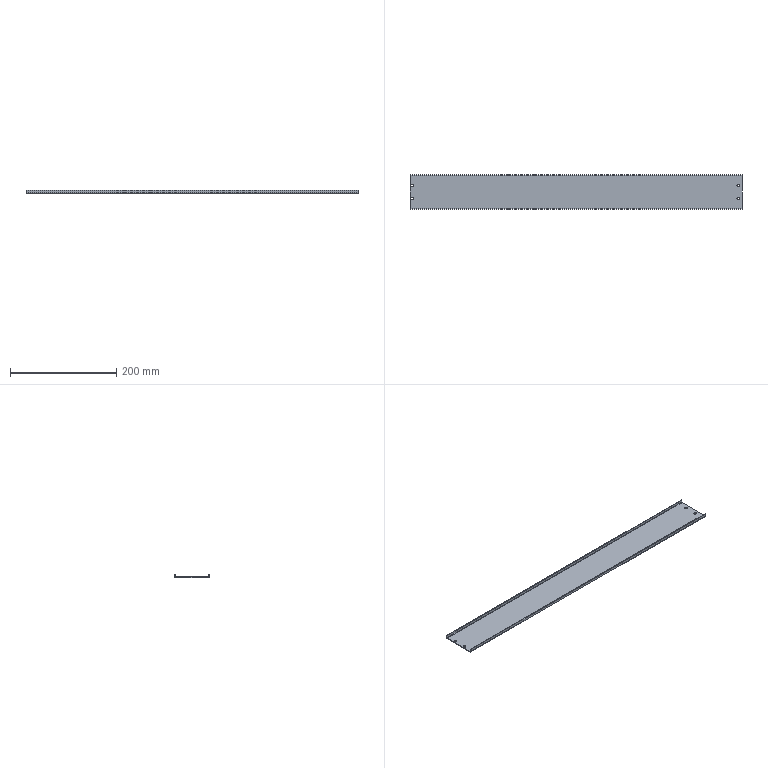Part | NX | features BREP 1 | 1 solid | 30 faces | box 625 x 65 x 6.5 mm | volume 68998 mm3 | plane 18 | cylinder 12 | commonest cylinder face diameters 5 x8 1.473 x2 4.473 x2
STEP:
#1=CARTESIAN_POINT('',(303.,-12.,0.));
#2=VERTEX_POINT('',#1);
#3=CARTESIAN_POINT('',(308.,-12.,0.));
#4=VERTEX_POINT('',#3);
#5=CARTESIAN_POINT('',(305.5,-12.,0.));
#6=DIRECTION('',(0.,0.,1.));
#7=DIRECTION('',(1.,0.,0.));
#8=AXIS2_PLACEMENT_3D('',#5,#6,#7);
#9=CIRCLE('',#8,2.5);
#10=EDGE_CURVE('',#2,#4,#9,.T.);
#11=ORIENTED_EDGE('',*,*,#10,.T.);
#12=CARTESIAN_POINT('',(308.,-12.,-1.5));
#13=VERTEX_POINT('',#12);
#14=CARTESIAN_POINT('',(308.,-12.,8.5));
#15=DIRECTION('',(0.,0.,-1.));
#16=VECTOR('',#15,1000.);
#17=LINE('',#14,#16);
#18=EDGE_CURVE('',#4,#13,#17,.T.);
#19=ORIENTED_EDGE('',*,*,#18,.T.);
#20=CARTESIAN_POINT('',(303.,-12.,-1.5));
#21=VERTEX_POINT('',#20);
#22=CARTESIAN_POINT('',(305.5,-12.,-1.5));
#23=DIRECTION('',(0.,0.,-1.));
#24=DIRECTION('',(-1.,0.,0.));
#25=AXIS2_PLACEMENT_3D('',#22,#23,#24);
#26=CIRCLE('',#25,2.5);
#27=EDGE_CURVE('',#13,#21,#26,.T.);
#28=ORIENTED_EDGE('',*,*,#27,.T.);
#29=CARTESIAN_POINT('',(303.,-12.,8.5));
#30=DIRECTION('',(0.,0.,-1.));
#31=VECTOR('',#30,1000.);
#32=LINE('',#29,#31);
#33=EDGE_CURVE('',#2,#21,#32,.T.);
#34=ORIENTED_EDGE('',*,*,#33,.F.);
#35=EDGE_LOOP('',(#11,#19,#28,#34));
#36=FACE_BOUND('',#35,.T.);
#37=CARTESIAN_POINT('',(305.5,-12.,8.5));
#38=DIRECTION('',(0.,0.,-1.));
#39=DIRECTION('',(-1.,0.,0.));
#40=AXIS2_PLACEMENT_3D('',#37,#38,#39);
#41=CYLINDRICAL_SURFACE('',#40,2.5);
#42=ADVANCED_FACE('',(#36),#41,.F.);
#43=CARTESIAN_POINT('',(303.,12.,0.));
#44=VERTEX_POINT('',#43);
#45=CARTESIAN_POINT('',(308.,12.,0.));
#46=VERTEX_POINT('',#45);
#47=CARTESIAN_POINT('',(305.5,12.,0.));
#48=DIRECTION('',(0.,0.,1.));
#49=DIRECTION('',(1.,0.,0.));
#50=AXIS2_PLACEMENT_3D('',#47,#48,#49);
#51=CIRCLE('',#50,2.5);
#52=EDGE_CURVE('',#44,#46,#51,.T.);
#53=ORIENTED_EDGE('',*,*,#52,.T.);
#54=CARTESIAN_POINT('',(308.,12.,-1.5));
#55=VERTEX_POINT('',#54);
#56=CARTESIAN_POINT('',(308.,12.,8.5));
#57=DIRECTION('',(0.,0.,-1.));
#58=VECTOR('',#57,1000.);
#59=LINE('',#56,#58);
#60=EDGE_CURVE('',#46,#55,#59,.T.);
#61=ORIENTED_EDGE('',*,*,#60,.T.);
#62=CARTESIAN_POINT('',(303.,12.,-1.5));
#63=VERTEX_POINT('',#62);
#64=CARTESIAN_POINT('',(305.5,12.,-1.5));
#65=DIRECTION('',(0.,0.,-1.));
#66=DIRECTION('',(-1.,0.,0.));
#67=AXIS2_PLACEMENT_3D('',#64,#65,#66);
#68=CIRCLE('',#67,2.5);
#69=EDGE_CURVE('',#55,#63,#68,.T.);
#70=ORIENTED_EDGE('',*,*,#69,.T.);
#71=CARTESIAN_POINT('',(303.,12.,8.5));
#72=DIRECTION('',(0.,0.,-1.));
#73=VECTOR('',#72,1000.);
#74=LINE('',#71,#73);
#75=EDGE_CURVE('',#44,#63,#74,.T.);
#76=ORIENTED_EDGE('',*,*,#75,.F.);
#77=EDGE_LOOP('',(#53,#61,#70,#76));
#78=FACE_BOUND('',#77,.T.);
#79=CARTESIAN_POINT('',(305.5,12.,8.5));
#80=DIRECTION('',(0.,0.,-1.));
#81=DIRECTION('',(-1.,0.,0.));
#82=AXIS2_PLACEMENT_3D('',#79,#80,#81);
#83=CYLINDRICAL_SURFACE('',#82,2.5);
#84=ADVANCED_FACE('',(#78),#83,.F.);
#85=CARTESIAN_POINT('',(-311.,-12.,0.));
#86=VERTEX_POINT('',#85);
#87=CARTESIAN_POINT('',(-306.,-12.,0.));
#88=VERTEX_POINT('',#87);
#89=CARTESIAN_POINT('',(-308.5,-12.,0.));
#90=DIRECTION('',(0.,0.,1.));
#91=DIRECTION('',(1.,0.,0.));
#92=AXIS2_PLACEMENT_3D('',#89,#90,#91);
#93=CIRCLE('',#92,2.5);
#94=EDGE_CURVE('',#86,#88,#93,.T.);
#95=ORIENTED_EDGE('',*,*,#94,.T.);
#96=CARTESIAN_POINT('',(-306.,-12.,-1.5));
#97=VERTEX_POINT('',#96);
#98=CARTESIAN_POINT('',(-306.,-12.,8.5));
#99=DIRECTION('',(0.,0.,-1.));
#100=VECTOR('',#99,1000.);
#101=LINE('',#98,#100);
#102=EDGE_CURVE('',#88,#97,#101,.T.);
#103=ORIENTED_EDGE('',*,*,#102,.T.);
#104=CARTESIAN_POINT('',(-311.,-12.,-1.5));
#105=VERTEX_POINT('',#104);
#106=CARTESIAN_POINT('',(-308.5,-12.,-1.5));
#107=DIRECTION('',(0.,0.,-1.));
#108=DIRECTION('',(-1.,0.,0.));
#109=AXIS2_PLACEMENT_3D('',#106,#107,#108);
#110=CIRCLE('',#109,2.5);
#111=EDGE_CURVE('',#97,#105,#110,.T.);
#112=ORIENTED_EDGE('',*,*,#111,.T.);
#113=CARTESIAN_POINT('',(-311.,-12.,8.5));
#114=DIRECTION('',(0.,0.,-1.));
#115=VECTOR('',#114,1000.);
#116=LINE('',#113,#115);
#117=EDGE_CURVE('',#86,#105,#116,.T.);
#118=ORIENTED_EDGE('',*,*,#117,.F.);
#119=EDGE_LOOP('',(#95,#103,#112,#118));
#120=FACE_BOUND('',#119,.T.);
#121=CARTESIAN_POINT('',(-308.5,-12.,8.5));
#122=DIRECTION('',(0.,0.,-1.));
#123=DIRECTION('',(-1.,0.,0.));
#124=AXIS2_PLACEMENT_3D('',#121,#122,#123);
#125=CYLINDRICAL_SURFACE('',#124,2.5);
#126=ADVANCED_FACE('',(#120),#125,.F.);
#127=CARTESIAN_POINT('',(-311.,12.,0.));
#128=VERTEX_POINT('',#127);
#129=CARTESIAN_POINT('',(-306.,12.,0.));
#130=VERTEX_POINT('',#129);
#131=CARTESIAN_POINT('',(-308.5,12.,0.));
#132=DIRECTION('',(0.,0.,1.));
#133=DIRECTION('',(1.,0.,0.));
#134=AXIS2_PLACEMENT_3D('',#131,#132,#133);
#135=CIRCLE('',#134,2.5);
#136=EDGE_CURVE('',#128,#130,#135,.T.);
#137=ORIENTED_EDGE('',*,*,#136,.T.);
#138=CARTESIAN_POINT('',(-306.,12.,-1.5));
#139=VERTEX_POINT('',#138);
#140=CARTESIAN_POINT('',(-306.,12.,8.5));
#141=DIRECTION('',(0.,0.,-1.));
#142=VECTOR('',#141,1000.);
#143=LINE('',#140,#142);
#144=EDGE_CURVE('',#130,#139,#143,.T.);
#145=ORIENTED_EDGE('',*,*,#144,.T.);
#146=CARTESIAN_POINT('',(-311.,12.,-1.5));
#147=VERTEX_POINT('',#146);
#148=CARTESIAN_POINT('',(-308.5,12.,-1.5));
#149=DIRECTION('',(0.,0.,-1.));
#150=DIRECTION('',(-1.,0.,0.));
#151=AXIS2_PLACEMENT_3D('',#148,#149,#150);
#152=CIRCLE('',#151,2.5);
#153=EDGE_CURVE('',#139,#147,#152,.T.);
#154=ORIENTED_EDGE('',*,*,#153,.T.);
#155=CARTESIAN_POINT('',(-311.,12.,8.5));
#156=DIRECTION('',(0.,0.,-1.));
#157=VECTOR('',#156,1000.);
#158=LINE('',#155,#157);
#159=EDGE_CURVE('',#128,#147,#158,.T.);
#160=ORIENTED_EDGE('',*,*,#159,.F.);
#161=EDGE_LOOP('',(#137,#145,#154,#160));
#162=FACE_BOUND('',#161,.T.);
#163=CARTESIAN_POINT('',(-308.5,12.,8.5));
#164=DIRECTION('',(0.,0.,-1.));
#165=DIRECTION('',(-1.,0.,0.));
#166=AXIS2_PLACEMENT_3D('',#163,#164,#165);
#167=CYLINDRICAL_SURFACE('',#166,2.5);
#168=ADVANCED_FACE('',(#162),#167,.F.);
#169=CARTESIAN_POINT('',(312.5,-30.263,-1.5));
#170=VERTEX_POINT('',#169);
#171=CARTESIAN_POINT('',(-312.5,-30.263,-1.5));
#172=VERTEX_POINT('',#171);
#173=CARTESIAN_POINT('',(312.5,-30.263,-1.5));
#174=DIRECTION('',(-1.,0.,0.));
#175=VECTOR('',#174,1000.);
#176=LINE('',#173,#175);
#177=EDGE_CURVE('',#170,#172,#176,.T.);
#178=ORIENTED_EDGE('',*,*,#177,.T.);
#179=CARTESIAN_POINT('',(-312.5,30.263,-1.5));
#180=VERTEX_POINT('',#179);
#181=CARTESIAN_POINT('',(-312.5,31.,-1.5));
#182=DIRECTION('',(0.,-1.,0.));
#183=VECTOR('',#182,1000.);
#184=LINE('',#181,#183);
#185=EDGE_CURVE('',#180,#172,#184,.T.);
#186=ORIENTED_EDGE('',*,*,#185,.F.);
#187=CARTESIAN_POINT('',(312.5,30.263,-1.5));
#188=VERTEX_POINT('',#187);
#189=CARTESIAN_POINT('',(-312.5,30.263,-1.5));
#190=DIRECTION('',(1.,0.,0.));
#191=VECTOR('',#190,1000.);
#192=LINE('',#189,#191);
#193=EDGE_CURVE('',#180,#188,#192,.T.);
#194=ORIENTED_EDGE('',*,*,#193,.T.);
#195=CARTESIAN_POINT('',(312.5,31.,-1.5));
#196=DIRECTION('',(0.,1.,0.));
#197=VECTOR('',#196,1000.);
#198=LINE('',#195,#197);
#199=EDGE_CURVE('',#170,#188,#198,.T.);
#200=ORIENTED_EDGE('',*,*,#199,.F.);
#201=EDGE_LOOP('',(#178,#186,#194,#200));
#202=FACE_BOUND('',#201,.T.);
#203=CARTESIAN_POINT('',(305.5,-12.,-1.5));
#204=DIRECTION('',(0.,0.,-1.));
#205=DIRECTION('',(-1.,0.,0.));
#206=AXIS2_PLACEMENT_3D('',#203,#204,#205);
#207=CIRCLE('',#206,2.5);
#208=EDGE_CURVE('',#21,#13,#207,.T.);
#209=ORIENTED_EDGE('',*,*,#208,.F.);
#210=ORIENTED_EDGE('',*,*,#27,.F.);
#211=EDGE_LOOP('',(#209,#210));
#212=FACE_BOUND('',#211,.T.);
#213=CARTESIAN_POINT('',(305.5,12.,-1.5));
#214=DIRECTION('',(0.,0.,-1.));
#215=DIRECTION('',(-1.,0.,0.));
#216=AXIS2_PLACEMENT_3D('',#213,#214,#215);
#217=CIRCLE('',#216,2.5);
#218=EDGE_CURVE('',#63,#55,#217,.T.);
#219=ORIENTED_EDGE('',*,*,#218,.F.);
#220=ORIENTED_EDGE('',*,*,#69,.F.);
#221=EDGE_LOOP('',(#219,#220));
#222=FACE_BOUND('',#221,.T.);
#223=CARTESIAN_POINT('',(-308.5,-12.,-1.5));
#224=DIRECTION('',(0.,0.,-1.));
#225=DIRECTION('',(-1.,0.,0.));
#226=AXIS2_PLACEMENT_3D('',#223,#224,#225);
#227=CIRCLE('',#226,2.5);
#228=EDGE_CURVE('',#105,#97,#227,.T.);
#229=ORIENTED_EDGE('',*,*,#228,.F.);
#230=ORIENTED_EDGE('',*,*,#111,.F.);
#231=EDGE_LOOP('',(#229,#230));
#232=FACE_BOUND('',#231,.T.);
#233=CARTESIAN_POINT('',(-308.5,12.,-1.5));
#234=DIRECTION('',(0.,0.,-1.));
#235=DIRECTION('',(-1.,0.,0.));
#236=AXIS2_PLACEMENT_3D('',#233,#234,#235);
#237=CIRCLE('',#236,2.5);
#238=EDGE_CURVE('',#147,#139,#237,.T.);
#239=ORIENTED_EDGE('',*,*,#238,.F.);
#240=ORIENTED_EDGE('',*,*,#153,.F.);
#241=EDGE_LOOP('',(#239,#240));
#242=FACE_BOUND('',#241,.T.);
#243=CARTESIAN_POINT('',(0.,0.,-1.5));
#244=DIRECTION('',(0.,0.,1.));
#245=DIRECTION('',(1.,0.,0.));
#246=AXIS2_PLACEMENT_3D('',#243,#244,#245);
#247=PLANE('',#246);
#248=ADVANCED_FACE('',(#202,#212,#222,#232,#242),#247,.F.);
#249=CARTESIAN_POINT('',(-312.5,30.263,0.));
#250=VERTEX_POINT('',#249);
#251=CARTESIAN_POINT('',(-312.5,-30.263,0.));
#252=VERTEX_POINT('',#251);
#253=CARTESIAN_POINT('',(-312.5,31.,0.));
#254=DIRECTION('',(0.,-1.,0.));
#255=VECTOR('',#254,1000.);
#256=LINE('',#253,#255);
#257=EDGE_CURVE('',#250,#252,#256,.T.);
#258=ORIENTED_EDGE('',*,*,#257,.T.);
#259=CARTESIAN_POINT('',(312.5,-30.263,0.));
#260=VERTEX_POINT('',#259);
#261=CARTESIAN_POINT('',(312.5,-30.263,0.));
#262=DIRECTION('',(-1.,0.,0.));
#263=VECTOR('',#262,1000.);
#264=LINE('',#261,#263);
#265=EDGE_CURVE('',#260,#252,#264,.T.);
#266=ORIENTED_EDGE('',*,*,#265,.F.);
#267=CARTESIAN_POINT('',(312.5,30.263,0.));
#268=VERTEX_POINT('',#267);
#269=CARTESIAN_POINT('',(312.5,31.,0.));
#270=DIRECTION('',(0.,1.,0.));
#271=VECTOR('',#270,1000.);
#272=LINE('',#269,#271);
#273=EDGE_CURVE('',#260,#268,#272,.T.);
#274=ORIENTED_EDGE('',*,*,#273,.T.);
#275=CARTESIAN_POINT('',(-312.5,30.263,0.));
#276=DIRECTION('',(1.,0.,0.));
#277=VECTOR('',#276,1000.);
#278=LINE('',#275,#277);
#279=EDGE_CURVE('',#250,#268,#278,.T.);
#280=ORIENTED_EDGE('',*,*,#279,.F.);
#281=EDGE_LOOP('',(#258,#266,#274,#280));
#282=FACE_BOUND('',#281,.T.);
#283=ORIENTED_EDGE('',*,*,#10,.F.);
#284=CARTESIAN_POINT('',(305.5,-12.,0.));
#285=DIRECTION('',(0.,0.,1.));
#286=DIRECTION('',(1.,0.,0.));
#287=AXIS2_PLACEMENT_3D('',#284,#285,#286);
#288=CIRCLE('',#287,2.5);
#289=EDGE_CURVE('',#4,#2,#288,.T.);
#290=ORIENTED_EDGE('',*,*,#289,.F.);
#291=EDGE_LOOP('',(#283,#290));
#292=FACE_BOUND('',#291,.T.);
#293=ORIENTED_EDGE('',*,*,#52,.F.);
#294=CARTESIAN_POINT('',(305.5,12.,0.));
#295=DIRECTION('',(0.,0.,1.));
#296=DIRECTION('',(1.,0.,0.));
#297=AXIS2_PLACEMENT_3D('',#294,#295,#296);
#298=CIRCLE('',#297,2.5);
#299=EDGE_CURVE('',#46,#44,#298,.T.);
#300=ORIENTED_EDGE('',*,*,#299,.F.);
#301=EDGE_LOOP('',(#293,#300));
#302=FACE_BOUND('',#301,.T.);
#303=ORIENTED_EDGE('',*,*,#94,.F.);
#304=CARTESIAN_POINT('',(-308.5,-12.,0.));
#305=DIRECTION('',(0.,0.,1.));
#306=DIRECTION('',(1.,0.,0.));
#307=AXIS2_PLACEMENT_3D('',#304,#305,#306);
#308=CIRCLE('',#307,2.5);
#309=EDGE_CURVE('',#88,#86,#308,.T.);
#310=ORIENTED_EDGE('',*,*,#309,.F.);
#311=EDGE_LOOP('',(#303,#310));
#312=FACE_BOUND('',#311,.T.);
#313=ORIENTED_EDGE('',*,*,#136,.F.);
#314=CARTESIAN_POINT('',(-308.5,12.,0.));
#315=DIRECTION('',(0.,0.,1.));
#316=DIRECTION('',(1.,0.,0.));
#317=AXIS2_PLACEMENT_3D('',#314,#315,#316);
#318=CIRCLE('',#317,2.5);
#319=EDGE_CURVE('',#130,#128,#318,.T.);
#320=ORIENTED_EDGE('',*,*,#319,.F.);
#321=EDGE_LOOP('',(#313,#320));
#322=FACE_BOUND('',#321,.T.);
#323=CARTESIAN_POINT('',(0.,0.,0.));
#324=DIRECTION('',(0.,0.,1.));
#325=DIRECTION('',(1.,0.,0.));
#326=AXIS2_PLACEMENT_3D('',#323,#324,#325);
#327=PLANE('',#326);
#328=ADVANCED_FACE('',(#282,#292,#302,#312,#322),#327,.T.);
#329=ORIENTED_EDGE('',*,*,#273,.F.);
#330=CARTESIAN_POINT('',(312.5,-30.263,0.));
#331=DIRECTION('',(0.,0.,-1.));
#332=VECTOR('',#331,1000.);
#333=LINE('',#330,#332);
#334=EDGE_CURVE('',#260,#170,#333,.T.);
#335=ORIENTED_EDGE('',*,*,#334,.T.);
#336=ORIENTED_EDGE('',*,*,#199,.T.);
#337=CARTESIAN_POINT('',(312.5,30.263,0.));
#338=DIRECTION('',(0.,0.,-1.));
#339=VECTOR('',#338,1000.);
#340=LINE('',#337,#339);
#341=EDGE_CURVE('',#268,#188,#340,.T.);
#342=ORIENTED_EDGE('',*,*,#341,.F.);
#343=EDGE_LOOP('',(#329,#335,#336,#342));
#344=FACE_BOUND('',#343,.T.);
#345=CARTESIAN_POINT('',(312.5,31.,-1.5));
#346=DIRECTION('',(1.,0.,0.));
#347=DIRECTION('',(0.,1.,0.));
#348=AXIS2_PLACEMENT_3D('',#345,#346,#347);
#349=PLANE('',#348);
#350=ADVANCED_FACE('',(#344),#349,.T.);
#351=CARTESIAN_POINT('',(-312.5,-30.263,0.));
#352=DIRECTION('',(0.,0.,-1.));
#353=VECTOR('',#352,1000.);
#354=LINE('',#351,#353);
#355=EDGE_CURVE('',#252,#172,#354,.T.);
#356=ORIENTED_EDGE('',*,*,#355,.F.);
#357=ORIENTED_EDGE('',*,*,#257,.F.);
#358=CARTESIAN_POINT('',(-312.5,30.263,0.));
#359=DIRECTION('',(0.,0.,-1.));
#360=VECTOR('',#359,1000.);
#361=LINE('',#358,#360);
#362=EDGE_CURVE('',#250,#180,#361,.T.);
#363=ORIENTED_EDGE('',*,*,#362,.T.);
#364=ORIENTED_EDGE('',*,*,#185,.T.);
#365=EDGE_LOOP('',(#356,#357,#363,#364));
#366=FACE_BOUND('',#365,.T.);
#367=CARTESIAN_POINT('',(-312.5,31.,-1.5));
#368=DIRECTION('',(-1.,0.,0.));
#369=DIRECTION('',(0.,0.,1.));
#370=AXIS2_PLACEMENT_3D('',#367,#368,#369);
#371=PLANE('',#370);
#372=ADVANCED_FACE('',(#366),#371,.T.);
#373=CARTESIAN_POINT('',(312.5,31.,0.7366));
#374=VERTEX_POINT('',#373);
#375=CARTESIAN_POINT('',(312.5,32.5,0.7366));
#376=VERTEX_POINT('',#375);
#377=CARTESIAN_POINT('',(312.5,31.,0.7366));
#378=DIRECTION('',(0.,1.,0.));
#379=VECTOR('',#378,1000.);
#380=LINE('',#377,#379);
#381=EDGE_CURVE('',#374,#376,#380,.T.);
#382=ORIENTED_EDGE('',*,*,#381,.F.);
#383=CARTESIAN_POINT('',(312.5,30.263,0.7366));
#384=DIRECTION('',(1.,0.,0.));
#385=DIRECTION('',(0.,0.,1.));
#386=AXIS2_PLACEMENT_3D('',#383,#384,#385);
#387=CIRCLE('',#386,0.7366);
#388=EDGE_CURVE('',#268,#374,#387,.T.);
#389=ORIENTED_EDGE('',*,*,#388,.F.);
#390=ORIENTED_EDGE('',*,*,#341,.T.);
#391=CARTESIAN_POINT('',(312.5,30.263,0.7366));
#392=DIRECTION('',(1.,0.,0.));
#393=DIRECTION('',(0.,0.,1.));
#394=AXIS2_PLACEMENT_3D('',#391,#392,#393);
#395=CIRCLE('',#394,2.237);
#396=EDGE_CURVE('',#188,#376,#395,.T.);
#397=ORIENTED_EDGE('',*,*,#396,.T.);
#398=EDGE_LOOP('',(#382,#389,#390,#397));
#399=FACE_BOUND('',#398,.T.);
#400=CARTESIAN_POINT('',(312.5,30.263,0.7366));
#401=DIRECTION('',(1.,0.,0.));
#402=DIRECTION('',(0.,1.,0.));
#403=AXIS2_PLACEMENT_3D('',#400,#401,#402);
#404=PLANE('',#403);
#405=ADVANCED_FACE('',(#399),#404,.T.);
#406=CARTESIAN_POINT('',(-312.5,31.,0.7366));
#407=VERTEX_POINT('',#406);
#408=CARTESIAN_POINT('',(-312.5,30.263,0.7366));
#409=DIRECTION('',(-1.,0.,0.));
#410=DIRECTION('',(0.,0.,1.));
#411=AXIS2_PLACEMENT_3D('',#408,#409,#410);
#412=CIRCLE('',#411,0.7366);
#413=EDGE_CURVE('',#407,#250,#412,.T.);
#414=ORIENTED_EDGE('',*,*,#413,.F.);
#415=CARTESIAN_POINT('',(-312.5,32.5,0.7366));
#416=VERTEX_POINT('',#415);
#417=CARTESIAN_POINT('',(-312.5,31.,0.7366));
#418=DIRECTION('',(0.,1.,0.));
#419=VECTOR('',#418,1000.);
#420=LINE('',#417,#419);
#421=EDGE_CURVE('',#407,#416,#420,.T.);
#422=ORIENTED_EDGE('',*,*,#421,.T.);
#423=CARTESIAN_POINT('',(-312.5,30.263,0.7366));
#424=DIRECTION('',(-1.,0.,0.));
#425=DIRECTION('',(0.,0.,1.));
#426=AXIS2_PLACEMENT_3D('',#423,#424,#425);
#427=CIRCLE('',#426,2.237);
#428=EDGE_CURVE('',#416,#180,#427,.T.);
#429=ORIENTED_EDGE('',*,*,#428,.T.);
#430=ORIENTED_EDGE('',*,*,#362,.F.);
#431=EDGE_LOOP('',(#414,#422,#429,#430));
#432=FACE_BOUND('',#431,.T.);
#433=CARTESIAN_POINT('',(-312.5,30.263,0.7366));
#434=DIRECTION('',(1.,0.,0.));
#435=DIRECTION('',(0.,1.,0.));
#436=AXIS2_PLACEMENT_3D('',#433,#434,#435);
#437=PLANE('',#436);
#438=ADVANCED_FACE('',(#432),#437,.F.);
#439=ORIENTED_EDGE('',*,*,#193,.F.);
#440=ORIENTED_EDGE('',*,*,#428,.F.);
#441=CARTESIAN_POINT('',(0.,32.5,0.7366));
#442=DIRECTION('',(-1.,0.,0.));
#443=VECTOR('',#442,1000.);
#444=LINE('',#441,#443);
#445=EDGE_CURVE('',#376,#416,#444,.T.);
#446=ORIENTED_EDGE('',*,*,#445,.F.);
#447=ORIENTED_EDGE('',*,*,#396,.F.);
#448=EDGE_LOOP('',(#439,#440,#446,#447));
#449=FACE_BOUND('',#448,.T.);
#450=CARTESIAN_POINT('',(-312.5,30.263,0.7366));
#451=DIRECTION('',(-1.,0.,0.));
#452=DIRECTION('',(0.,1.,0.));
#453=AXIS2_PLACEMENT_3D('',#450,#451,#452);
#454=CYLINDRICAL_SURFACE('',#453,2.237);
#455=ADVANCED_FACE('',(#449),#454,.T.);
#456=ORIENTED_EDGE('',*,*,#279,.T.);
#457=ORIENTED_EDGE('',*,*,#388,.T.);
#458=CARTESIAN_POINT('',(312.5,31.,0.7366));
#459=DIRECTION('',(-1.,0.,0.));
#460=VECTOR('',#459,1000.);
#461=LINE('',#458,#460);
#462=EDGE_CURVE('',#374,#407,#461,.T.);
#463=ORIENTED_EDGE('',*,*,#462,.T.);
#464=ORIENTED_EDGE('',*,*,#413,.T.);
#465=EDGE_LOOP('',(#456,#457,#463,#464));
#466=FACE_BOUND('',#465,.T.);
#467=CARTESIAN_POINT('',(-312.5,30.263,0.7366));
#468=DIRECTION('',(-1.,0.,0.));
#469=DIRECTION('',(0.,1.,0.));
#470=AXIS2_PLACEMENT_3D('',#467,#468,#469);
#471=CYLINDRICAL_SURFACE('',#470,0.7366);
#472=ADVANCED_FACE('',(#466),#471,.F.);
#473=CARTESIAN_POINT('',(-312.5,32.5,5.));
#474=VERTEX_POINT('',#473);
#475=CARTESIAN_POINT('',(-312.5,32.5,0.));
#476=DIRECTION('',(0.,0.,-1.));
#477=VECTOR('',#476,1000.);
#478=LINE('',#475,#477);
#479=EDGE_CURVE('',#474,#416,#478,.T.);
#480=ORIENTED_EDGE('',*,*,#479,.T.);
#481=ORIENTED_EDGE('',*,*,#421,.F.);
#482=CARTESIAN_POINT('',(-312.5,31.,5.));
#483=VERTEX_POINT('',#482);
#484=CARTESIAN_POINT('',(-312.5,31.,0.));
#485=DIRECTION('',(0.,0.,-1.));
#486=VECTOR('',#485,1000.);
#487=LINE('',#484,#486);
#488=EDGE_CURVE('',#483,#407,#487,.T.);
#489=ORIENTED_EDGE('',*,*,#488,.F.);
#490=CARTESIAN_POINT('',(-312.5,32.5,5.));
#491=DIRECTION('',(0.,-1.,0.));
#492=VECTOR('',#491,1000.);
#493=LINE('',#490,#492);
#494=EDGE_CURVE('',#474,#483,#493,.T.);
#495=ORIENTED_EDGE('',*,*,#494,.F.);
#496=EDGE_LOOP('',(#480,#481,#489,#495));
#497=FACE_BOUND('',#496,.T.);
#498=CARTESIAN_POINT('',(-312.5,32.5,0.));
#499=DIRECTION('',(-1.,0.,0.));
#500=DIRECTION('',(0.,0.,1.));
#501=AXIS2_PLACEMENT_3D('',#498,#499,#500);
#502=PLANE('',#501);
#503=ADVANCED_FACE('',(#497),#502,.T.);
#504=CARTESIAN_POINT('',(312.5,31.,5.));
#505=VERTEX_POINT('',#504);
#506=CARTESIAN_POINT('',(312.5,31.,5.));
#507=DIRECTION('',(0.,0.,1.));
#508=VECTOR('',#507,1000.);
#509=LINE('',#506,#508);
#510=EDGE_CURVE('',#374,#505,#509,.T.);
#511=ORIENTED_EDGE('',*,*,#510,.F.);
#512=ORIENTED_EDGE('',*,*,#381,.T.);
#513=CARTESIAN_POINT('',(312.5,32.5,5.));
#514=VERTEX_POINT('',#513);
#515=CARTESIAN_POINT('',(312.5,32.5,5.));
#516=DIRECTION('',(0.,0.,1.));
#517=VECTOR('',#516,1000.);
#518=LINE('',#515,#517);
#519=EDGE_CURVE('',#376,#514,#518,.T.);
#520=ORIENTED_EDGE('',*,*,#519,.T.);
#521=CARTESIAN_POINT('',(312.5,32.5,5.));
#522=DIRECTION('',(0.,-1.,0.));
#523=VECTOR('',#522,1000.);
#524=LINE('',#521,#523);
#525=EDGE_CURVE('',#514,#505,#524,.T.);
#526=ORIENTED_EDGE('',*,*,#525,.T.);
#527=EDGE_LOOP('',(#511,#512,#520,#526));
#528=FACE_BOUND('',#527,.T.);
#529=CARTESIAN_POINT('',(312.5,32.5,5.));
#530=DIRECTION('',(1.,0.,0.));
#531=DIRECTION('',(0.,1.,0.));
#532=AXIS2_PLACEMENT_3D('',#529,#530,#531);
#533=PLANE('',#532);
#534=ADVANCED_FACE('',(#528),#533,.T.);
#535=ORIENTED_EDGE('',*,*,#519,.F.);
#536=ORIENTED_EDGE('',*,*,#445,.T.);
#537=ORIENTED_EDGE('',*,*,#479,.F.);
#538=CARTESIAN_POINT('',(-312.5,32.5,5.));
#539=DIRECTION('',(-1.,0.,0.));
#540=VECTOR('',#539,1000.);
#541=LINE('',#538,#540);
#542=EDGE_CURVE('',#514,#474,#541,.T.);
#543=ORIENTED_EDGE('',*,*,#542,.F.);
#544=EDGE_LOOP('',(#535,#536,#537,#543));
#545=FACE_BOUND('',#544,.T.);
#546=CARTESIAN_POINT('',(0.,32.5,0.));
#547=DIRECTION('',(0.,1.,0.));
#548=DIRECTION('',(0.,0.,-1.));
#549=AXIS2_PLACEMENT_3D('',#546,#547,#548);
#550=PLANE('',#549);
#551=ADVANCED_FACE('',(#545),#550,.T.);
#552=ORIENTED_EDGE('',*,*,#462,.F.);
#553=ORIENTED_EDGE('',*,*,#510,.T.);
#554=CARTESIAN_POINT('',(-312.5,31.,5.));
#555=DIRECTION('',(-1.,0.,0.));
#556=VECTOR('',#555,1000.);
#557=LINE('',#554,#556);
#558=EDGE_CURVE('',#505,#483,#557,.T.);
#559=ORIENTED_EDGE('',*,*,#558,.T.);
#560=ORIENTED_EDGE('',*,*,#488,.T.);
#561=EDGE_LOOP('',(#552,#553,#559,#560));
#562=FACE_BOUND('',#561,.T.);
#563=CARTESIAN_POINT('',(0.,31.,0.));
#564=DIRECTION('',(0.,1.,0.));
#565=DIRECTION('',(0.,0.,-1.));
#566=AXIS2_PLACEMENT_3D('',#563,#564,#565);
#567=PLANE('',#566);
#568=ADVANCED_FACE('',(#562),#567,.F.);
#569=ORIENTED_EDGE('',*,*,#558,.F.);
#570=ORIENTED_EDGE('',*,*,#525,.F.);
#571=ORIENTED_EDGE('',*,*,#542,.T.);
#572=ORIENTED_EDGE('',*,*,#494,.T.);
#573=EDGE_LOOP('',(#569,#570,#571,#572));
#574=FACE_BOUND('',#573,.T.);
#575=CARTESIAN_POINT('',(-312.5,32.5,5.));
#576=DIRECTION('',(0.,0.,1.));
#577=DIRECTION('',(0.,-1.,0.));
#578=AXIS2_PLACEMENT_3D('',#575,#576,#577);
#579=PLANE('',#578);
#580=ADVANCED_FACE('',(#574),#579,.T.);
#581=CARTESIAN_POINT('',(-312.5,-31.,0.7366));
#582=VERTEX_POINT('',#581);
#583=CARTESIAN_POINT('',(-312.5,-32.5,0.7366));
#584=VERTEX_POINT('',#583);
#585=CARTESIAN_POINT('',(-312.5,-31.,0.7366));
#586=DIRECTION('',(0.,-1.,0.));
#587=VECTOR('',#586,1000.);
#588=LINE('',#585,#587);
#589=EDGE_CURVE('',#582,#584,#588,.T.);
#590=ORIENTED_EDGE('',*,*,#589,.F.);
#591=CARTESIAN_POINT('',(-312.5,-30.263,0.7366));
#592=DIRECTION('',(-1.,0.,0.));
#593=DIRECTION('',(0.,0.,-1.));
#594=AXIS2_PLACEMENT_3D('',#591,#592,#593);
#595=CIRCLE('',#594,0.7366);
#596=EDGE_CURVE('',#252,#582,#595,.T.);
#597=ORIENTED_EDGE('',*,*,#596,.F.);
#598=ORIENTED_EDGE('',*,*,#355,.T.);
#599=CARTESIAN_POINT('',(-312.5,-30.263,0.7366));
#600=DIRECTION('',(-1.,0.,0.));
#601=DIRECTION('',(0.,0.,-1.));
#602=AXIS2_PLACEMENT_3D('',#599,#600,#601);
#603=CIRCLE('',#602,2.237);
#604=EDGE_CURVE('',#172,#584,#603,.T.);
#605=ORIENTED_EDGE('',*,*,#604,.T.);
#606=EDGE_LOOP('',(#590,#597,#598,#605));
#607=FACE_BOUND('',#606,.T.);
#608=CARTESIAN_POINT('',(-312.5,-30.263,0.7366));
#609=DIRECTION('',(-1.,0.,0.));
#610=DIRECTION('',(0.,0.,1.));
#611=AXIS2_PLACEMENT_3D('',#608,#609,#610);
#612=PLANE('',#611);
#613=ADVANCED_FACE('',(#607),#612,.T.);
#614=CARTESIAN_POINT('',(312.5,-31.,0.7366));
#615=VERTEX_POINT('',#614);
#616=CARTESIAN_POINT('',(312.5,-30.263,0.7366));
#617=DIRECTION('',(1.,0.,0.));
#618=DIRECTION('',(0.,0.,-1.));
#619=AXIS2_PLACEMENT_3D('',#616,#617,#618);
#620=CIRCLE('',#619,0.7366);
#621=EDGE_CURVE('',#615,#260,#620,.T.);
#622=ORIENTED_EDGE('',*,*,#621,.F.);
#623=CARTESIAN_POINT('',(312.5,-32.5,0.7366));
#624=VERTEX_POINT('',#623);
#625=CARTESIAN_POINT('',(312.5,-31.,0.7366));
#626=DIRECTION('',(0.,-1.,0.));
#627=VECTOR('',#626,1000.);
#628=LINE('',#625,#627);
#629=EDGE_CURVE('',#615,#624,#628,.T.);
#630=ORIENTED_EDGE('',*,*,#629,.T.);
#631=CARTESIAN_POINT('',(312.5,-30.263,0.7366));
#632=DIRECTION('',(1.,0.,0.));
#633=DIRECTION('',(0.,0.,-1.));
#634=AXIS2_PLACEMENT_3D('',#631,#632,#633);
#635=CIRCLE('',#634,2.237);
#636=EDGE_CURVE('',#624,#170,#635,.T.);
#637=ORIENTED_EDGE('',*,*,#636,.T.);
#638=ORIENTED_EDGE('',*,*,#334,.F.);
#639=EDGE_LOOP('',(#622,#630,#637,#638));
#640=FACE_BOUND('',#639,.T.);
#641=CARTESIAN_POINT('',(312.5,-30.263,0.7366));
#642=DIRECTION('',(-1.,0.,0.));
#643=DIRECTION('',(0.,0.,1.));
#644=AXIS2_PLACEMENT_3D('',#641,#642,#643);
#645=PLANE('',#644);
#646=ADVANCED_FACE('',(#640),#645,.F.);
#647=ORIENTED_EDGE('',*,*,#177,.F.);
#648=ORIENTED_EDGE('',*,*,#636,.F.);
#649=CARTESIAN_POINT('',(0.,-32.5,0.7366));
#650=DIRECTION('',(-1.,0.,0.));
#651=VECTOR('',#650,1000.);
#652=LINE('',#649,#651);
#653=EDGE_CURVE('',#624,#584,#652,.T.);
#654=ORIENTED_EDGE('',*,*,#653,.T.);
#655=ORIENTED_EDGE('',*,*,#604,.F.);
#656=EDGE_LOOP('',(#647,#648,#654,#655));
#657=FACE_BOUND('',#656,.T.);
#658=CARTESIAN_POINT('',(312.5,-30.263,0.7366));
#659=DIRECTION('',(1.,0.,0.));
#660=DIRECTION('',(0.,-1.,0.));
#661=AXIS2_PLACEMENT_3D('',#658,#659,#660);
#662=CYLINDRICAL_SURFACE('',#661,2.237);
#663=ADVANCED_FACE('',(#657),#662,.T.);
#664=ORIENTED_EDGE('',*,*,#265,.T.);
#665=ORIENTED_EDGE('',*,*,#596,.T.);
#666=CARTESIAN_POINT('',(-312.5,-31.,0.7366));
#667=DIRECTION('',(1.,0.,0.));
#668=VECTOR('',#667,1000.);
#669=LINE('',#666,#668);
#670=EDGE_CURVE('',#582,#615,#669,.T.);
#671=ORIENTED_EDGE('',*,*,#670,.T.);
#672=ORIENTED_EDGE('',*,*,#621,.T.);
#673=EDGE_LOOP('',(#664,#665,#671,#672));
#674=FACE_BOUND('',#673,.T.);
#675=CARTESIAN_POINT('',(312.5,-30.263,0.7366));
#676=DIRECTION('',(1.,0.,0.));
#677=DIRECTION('',(0.,-1.,0.));
#678=AXIS2_PLACEMENT_3D('',#675,#676,#677);
#679=CYLINDRICAL_SURFACE('',#678,0.7366);
#680=ADVANCED_FACE('',(#674),#679,.F.);
#681=CARTESIAN_POINT('',(-312.5,-31.,5.));
#682=VERTEX_POINT('',#681);
#683=CARTESIAN_POINT('',(-312.5,-31.,0.));
#684=DIRECTION('',(0.,0.,1.));
#685=VECTOR('',#684,1000.);
#686=LINE('',#683,#685);
#687=EDGE_CURVE('',#582,#682,#686,.T.);
#688=ORIENTED_EDGE('',*,*,#687,.F.);
#689=ORIENTED_EDGE('',*,*,#589,.T.);
#690=CARTESIAN_POINT('',(-312.5,-32.5,5.));
#691=VERTEX_POINT('',#690);
#692=CARTESIAN_POINT('',(-312.5,-32.5,0.));
#693=DIRECTION('',(0.,0.,1.));
#694=VECTOR('',#693,1000.);
#695=LINE('',#692,#694);
#696=EDGE_CURVE('',#584,#691,#695,.T.);
#697=ORIENTED_EDGE('',*,*,#696,.T.);
#698=CARTESIAN_POINT('',(-312.5,-32.5,5.));
#699=DIRECTION('',(0.,1.,0.));
#700=VECTOR('',#699,1000.);
#701=LINE('',#698,#700);
#702=EDGE_CURVE('',#691,#682,#701,.T.);
#703=ORIENTED_EDGE('',*,*,#702,.T.);
#704=EDGE_LOOP('',(#688,#689,#697,#703));
#705=FACE_BOUND('',#704,.T.);
#706=CARTESIAN_POINT('',(-312.5,-32.5,0.));
#707=DIRECTION('',(-1.,0.,0.));
#708=DIRECTION('',(0.,0.,1.));
#709=AXIS2_PLACEMENT_3D('',#706,#707,#708);
#710=PLANE('',#709);
#711=ADVANCED_FACE('',(#705),#710,.T.);
#712=CARTESIAN_POINT('',(312.5,-32.5,5.));
#713=VERTEX_POINT('',#712);
#714=CARTESIAN_POINT('',(312.5,-32.5,5.));
#715=DIRECTION('',(0.,0.,-1.));
#716=VECTOR('',#715,1000.);
#717=LINE('',#714,#716);
#718=EDGE_CURVE('',#713,#624,#717,.T.);
#719=ORIENTED_EDGE('',*,*,#718,.T.);
#720=ORIENTED_EDGE('',*,*,#629,.F.);
#721=CARTESIAN_POINT('',(312.5,-31.,5.));
#722=VERTEX_POINT('',#721);
#723=CARTESIAN_POINT('',(312.5,-31.,5.));
#724=DIRECTION('',(0.,0.,-1.));
#725=VECTOR('',#724,1000.);
#726=LINE('',#723,#725);
#727=EDGE_CURVE('',#722,#615,#726,.T.);
#728=ORIENTED_EDGE('',*,*,#727,.F.);
#729=CARTESIAN_POINT('',(312.5,-32.5,5.));
#730=DIRECTION('',(0.,1.,0.));
#731=VECTOR('',#730,1000.);
#732=LINE('',#729,#731);
#733=EDGE_CURVE('',#713,#722,#732,.T.);
#734=ORIENTED_EDGE('',*,*,#733,.F.);
#735=EDGE_LOOP('',(#719,#720,#728,#734));
#736=FACE_BOUND('',#735,.T.);
#737=CARTESIAN_POINT('',(312.5,-32.5,5.));
#738=DIRECTION('',(1.,0.,0.));
#739=DIRECTION('',(0.,1.,0.));
#740=AXIS2_PLACEMENT_3D('',#737,#738,#739);
#741=PLANE('',#740);
#742=ADVANCED_FACE('',(#736),#741,.T.);
#743=ORIENTED_EDGE('',*,*,#653,.F.);
#744=ORIENTED_EDGE('',*,*,#718,.F.);
#745=CARTESIAN_POINT('',(-312.5,-32.5,5.));
#746=DIRECTION('',(1.,0.,0.));
#747=VECTOR('',#746,1000.);
#748=LINE('',#745,#747);
#749=EDGE_CURVE('',#691,#713,#748,.T.);
#750=ORIENTED_EDGE('',*,*,#749,.F.);
#751=ORIENTED_EDGE('',*,*,#696,.F.);
#752=EDGE_LOOP('',(#743,#744,#750,#751));
#753=FACE_BOUND('',#752,.T.);
#754=CARTESIAN_POINT('',(0.,-32.5,0.));
#755=DIRECTION('',(0.,1.,0.));
#756=DIRECTION('',(0.,0.,-1.));
#757=AXIS2_PLACEMENT_3D('',#754,#755,#756);
#758=PLANE('',#757);
#759=ADVANCED_FACE('',(#753),#758,.F.);
#760=ORIENTED_EDGE('',*,*,#727,.T.);
#761=ORIENTED_EDGE('',*,*,#670,.F.);
#762=ORIENTED_EDGE('',*,*,#687,.T.);
#763=CARTESIAN_POINT('',(-312.5,-31.,5.));
#764=DIRECTION('',(1.,0.,0.));
#765=VECTOR('',#764,1000.);
#766=LINE('',#763,#765);
#767=EDGE_CURVE('',#682,#722,#766,.T.);
#768=ORIENTED_EDGE('',*,*,#767,.T.);
#769=EDGE_LOOP('',(#760,#761,#762,#768));
#770=FACE_BOUND('',#769,.T.);
#771=CARTESIAN_POINT('',(0.,-31.,0.));
#772=DIRECTION('',(0.,1.,0.));
#773=DIRECTION('',(0.,0.,-1.));
#774=AXIS2_PLACEMENT_3D('',#771,#772,#773);
#775=PLANE('',#774);
#776=ADVANCED_FACE('',(#770),#775,.T.);
#777=ORIENTED_EDGE('',*,*,#767,.F.);
#778=ORIENTED_EDGE('',*,*,#702,.F.);
#779=ORIENTED_EDGE('',*,*,#749,.T.);
#780=ORIENTED_EDGE('',*,*,#733,.T.);
#781=EDGE_LOOP('',(#777,#778,#779,#780));
#782=FACE_BOUND('',#781,.T.);
#783=CARTESIAN_POINT('',(-312.5,-32.5,5.));
#784=DIRECTION('',(0.,0.,1.));
#785=DIRECTION('',(0.,-1.,0.));
#786=AXIS2_PLACEMENT_3D('',#783,#784,#785);
#787=PLANE('',#786);
#788=ADVANCED_FACE('',(#782),#787,.T.);
#789=ORIENTED_EDGE('',*,*,#144,.F.);
#790=ORIENTED_EDGE('',*,*,#319,.T.);
#791=ORIENTED_EDGE('',*,*,#159,.T.);
#792=ORIENTED_EDGE('',*,*,#238,.T.);
#793=EDGE_LOOP('',(#789,#790,#791,#792));
#794=FACE_BOUND('',#793,.T.);
#795=CARTESIAN_POINT('',(-308.5,12.,8.5));
#796=DIRECTION('',(0.,0.,-1.));
#797=DIRECTION('',(-1.,0.,0.));
#798=AXIS2_PLACEMENT_3D('',#795,#796,#797);
#799=CYLINDRICAL_SURFACE('',#798,2.5);
#800=ADVANCED_FACE('',(#794),#799,.F.);
#801=ORIENTED_EDGE('',*,*,#102,.F.);
#802=ORIENTED_EDGE('',*,*,#309,.T.);
#803=ORIENTED_EDGE('',*,*,#117,.T.);
#804=ORIENTED_EDGE('',*,*,#228,.T.);
#805=EDGE_LOOP('',(#801,#802,#803,#804));
#806=FACE_BOUND('',#805,.T.);
#807=CARTESIAN_POINT('',(-308.5,-12.,8.5));
#808=DIRECTION('',(0.,0.,-1.));
#809=DIRECTION('',(-1.,0.,0.));
#810=AXIS2_PLACEMENT_3D('',#807,#808,#809);
#811=CYLINDRICAL_SURFACE('',#810,2.5);
#812=ADVANCED_FACE('',(#806),#811,.F.);
#813=ORIENTED_EDGE('',*,*,#60,.F.);
#814=ORIENTED_EDGE('',*,*,#299,.T.);
#815=ORIENTED_EDGE('',*,*,#75,.T.);
#816=ORIENTED_EDGE('',*,*,#218,.T.);
#817=EDGE_LOOP('',(#813,#814,#815,#816));
#818=FACE_BOUND('',#817,.T.);
#819=CARTESIAN_POINT('',(305.5,12.,8.5));
#820=DIRECTION('',(0.,0.,-1.));
#821=DIRECTION('',(-1.,0.,0.));
#822=AXIS2_PLACEMENT_3D('',#819,#820,#821);
#823=CYLINDRICAL_SURFACE('',#822,2.5);
#824=ADVANCED_FACE('',(#818),#823,.F.);
#825=ORIENTED_EDGE('',*,*,#18,.F.);
#826=ORIENTED_EDGE('',*,*,#289,.T.);
#827=ORIENTED_EDGE('',*,*,#33,.T.);
#828=ORIENTED_EDGE('',*,*,#208,.T.);
#829=EDGE_LOOP('',(#825,#826,#827,#828));
#830=FACE_BOUND('',#829,.T.);
#831=CARTESIAN_POINT('',(305.5,-12.,8.5));
#832=DIRECTION('',(0.,0.,-1.));
#833=DIRECTION('',(-1.,0.,0.));
#834=AXIS2_PLACEMENT_3D('',#831,#832,#833);
#835=CYLINDRICAL_SURFACE('',#834,2.5);
#836=ADVANCED_FACE('',(#830),#835,.F.);
#837=CLOSED_SHELL('',(#42,#84,#126,#168,#248,#328,#350,#372,#405,#438,#455,#472,#503,#534,#551,#568,#580,#613,#646,#663,#680,#711,#742,#759,#776,#788,#800,#812,#824,#836));
#838=MANIFOLD_SOLID_BREP('',#837);
#839=(LENGTH_UNIT()NAMED_UNIT(*)SI_UNIT(.MILLI.,.METRE.));
#840=UNCERTAINTY_MEASURE_WITH_UNIT(LENGTH_MEASURE(0.00001),#839,'','');
#841=(NAMED_UNIT(*)PLANE_ANGLE_UNIT()SI_UNIT($,.RADIAN.));
#842=(NAMED_UNIT(*)SI_UNIT($,.STERADIAN.)SOLID_ANGLE_UNIT());
#843=(GEOMETRIC_REPRESENTATION_CONTEXT(3)GLOBAL_UNCERTAINTY_ASSIGNED_CONTEXT((#840))GLOBAL_UNIT_ASSIGNED_CONTEXT((#839,#841,#842))REPRESENTATION_CONTEXT('',''));
#844=ADVANCED_BREP_SHAPE_REPRESENTATION('',(#838),#843);